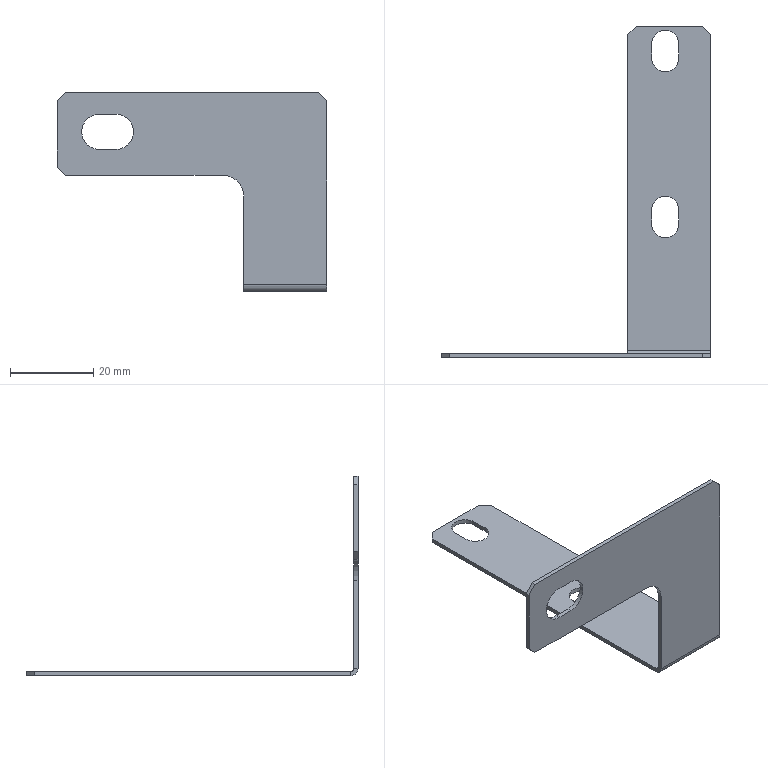Part | 1 solid | 34 faces | box 65 x 80 x 48 mm | volume 3222 mm3 | plane 25 | cylinder 9 | commonest cylinder face diameters 6.5 x4 8.5 x2 1.473 x1 3.473 x1 10 x1
STEP:
#1=CARTESIAN_POINT('',(45.,-1.,-46.263));
#2=VERTEX_POINT('',#1);
#3=CARTESIAN_POINT('',(45.,-1.,-25.));
#4=VERTEX_POINT('',#3);
#5=CARTESIAN_POINT('',(45.,-1.,-20.));
#6=DIRECTION('',(0.,0.,1.));
#7=VECTOR('',#6,1000.);
#8=LINE('',#5,#7);
#9=EDGE_CURVE('',#2,#4,#8,.T.);
#10=ORIENTED_EDGE('',*,*,#9,.T.);
#11=CARTESIAN_POINT('',(45.,0.,-25.));
#12=VERTEX_POINT('',#11);
#13=CARTESIAN_POINT('',(45.,0.,-25.));
#14=DIRECTION('',(0.,1.,0.));
#15=VECTOR('',#14,1000.);
#16=LINE('',#13,#15);
#17=EDGE_CURVE('',#4,#12,#16,.T.);
#18=ORIENTED_EDGE('',*,*,#17,.T.);
#19=CARTESIAN_POINT('',(45.,0.,-46.263));
#20=VERTEX_POINT('',#19);
#21=CARTESIAN_POINT('',(45.,0.,-20.));
#22=DIRECTION('',(0.,0.,1.));
#23=VECTOR('',#22,1000.);
#24=LINE('',#21,#23);
#25=EDGE_CURVE('',#20,#12,#24,.T.);
#26=ORIENTED_EDGE('',*,*,#25,.F.);
#27=CARTESIAN_POINT('',(45.,0.,-46.263));
#28=DIRECTION('',(0.,-1.,0.));
#29=VECTOR('',#28,1000.);
#30=LINE('',#27,#29);
#31=EDGE_CURVE('',#20,#2,#30,.T.);
#32=ORIENTED_EDGE('',*,*,#31,.T.);
#33=EDGE_LOOP('',(#10,#18,#26,#32));
#34=FACE_OUTER_BOUND('',#33,.T.);
#35=CARTESIAN_POINT('',(45.,-1.,-20.));
#36=DIRECTION('',(-1.,0.,0.));
#37=DIRECTION('',(0.,0.,1.));
#38=AXIS2_PLACEMENT_3D('',#35,#36,#37);
#39=PLANE('',#38);
#40=ADVANCED_FACE('',(#34),#39,.T.);
#41=CARTESIAN_POINT('',(10.164,-1.,-13.75));
#42=VERTEX_POINT('',#41);
#43=CARTESIAN_POINT('',(14.164,-1.,-13.75));
#44=VERTEX_POINT('',#43);
#45=CARTESIAN_POINT('',(10.164,-1.,-13.75));
#46=DIRECTION('',(1.,0.,0.));
#47=VECTOR('',#46,1000.);
#48=LINE('',#45,#47);
#49=EDGE_CURVE('',#42,#44,#48,.T.);
#50=ORIENTED_EDGE('',*,*,#49,.F.);
#51=CARTESIAN_POINT('',(10.164,-1.,-5.25));
#52=VERTEX_POINT('',#51);
#53=CARTESIAN_POINT('',(10.164,-1.,-9.5));
#54=DIRECTION('',(0.,1.,0.));
#55=DIRECTION('',(0.,0.,1.));
#56=AXIS2_PLACEMENT_3D('',#53,#54,#55);
#57=CIRCLE('',#56,4.25);
#58=EDGE_CURVE('',#42,#52,#57,.T.);
#59=ORIENTED_EDGE('',*,*,#58,.T.);
#60=CARTESIAN_POINT('',(14.164,-1.,-5.25));
#61=VERTEX_POINT('',#60);
#62=CARTESIAN_POINT('',(10.164,-1.,-5.25));
#63=DIRECTION('',(1.,0.,0.));
#64=VECTOR('',#63,1000.);
#65=LINE('',#62,#64);
#66=EDGE_CURVE('',#52,#61,#65,.T.);
#67=ORIENTED_EDGE('',*,*,#66,.T.);
#68=CARTESIAN_POINT('',(14.164,-1.,-9.5));
#69=DIRECTION('',(0.,1.,0.));
#70=DIRECTION('',(0.,0.,1.));
#71=AXIS2_PLACEMENT_3D('',#68,#69,#70);
#72=CIRCLE('',#71,4.25);
#73=EDGE_CURVE('',#61,#44,#72,.T.);
#74=ORIENTED_EDGE('',*,*,#73,.T.);
#75=EDGE_LOOP('',(#50,#59,#67,#74));
#76=FACE_BOUND('',#75,.T.);
#77=CARTESIAN_POINT('',(65.,-1.,-2.));
#78=VERTEX_POINT('',#77);
#79=CARTESIAN_POINT('',(65.,-1.,-46.263));
#80=VERTEX_POINT('',#79);
#81=CARTESIAN_POINT('',(65.,-1.,-48.));
#82=DIRECTION('',(0.,0.,-1.));
#83=VECTOR('',#82,1000.);
#84=LINE('',#81,#83);
#85=EDGE_CURVE('',#78,#80,#84,.T.);
#86=ORIENTED_EDGE('',*,*,#85,.F.);
#87=CARTESIAN_POINT('',(63.,-1.,0.));
#88=VERTEX_POINT('',#87);
#89=CARTESIAN_POINT('',(31.5,-1.,31.5));
#90=DIRECTION('',(-0.7071,0.,0.7071));
#91=VECTOR('',#90,1000.);
#92=LINE('',#89,#91);
#93=EDGE_CURVE('',#78,#88,#92,.T.);
#94=ORIENTED_EDGE('',*,*,#93,.T.);
#95=CARTESIAN_POINT('',(2.,-1.,0.));
#96=VERTEX_POINT('',#95);
#97=CARTESIAN_POINT('',(0.,-1.,0.));
#98=DIRECTION('',(1.,0.,0.));
#99=VECTOR('',#98,1000.);
#100=LINE('',#97,#99);
#101=EDGE_CURVE('',#96,#88,#100,.T.);
#102=ORIENTED_EDGE('',*,*,#101,.F.);
#103=CARTESIAN_POINT('',(0.,-1.,-2.));
#104=VERTEX_POINT('',#103);
#105=CARTESIAN_POINT('',(1.,-1.,-1.));
#106=DIRECTION('',(-0.7071,0.,-0.7071));
#107=VECTOR('',#106,1000.);
#108=LINE('',#105,#107);
#109=EDGE_CURVE('',#96,#104,#108,.T.);
#110=ORIENTED_EDGE('',*,*,#109,.T.);
#111=CARTESIAN_POINT('',(0.,-1.,-18.));
#112=VERTEX_POINT('',#111);
#113=CARTESIAN_POINT('',(0.,-1.,0.));
#114=DIRECTION('',(0.,0.,1.));
#115=VECTOR('',#114,1000.);
#116=LINE('',#113,#115);
#117=EDGE_CURVE('',#112,#104,#116,.T.);
#118=ORIENTED_EDGE('',*,*,#117,.F.);
#119=CARTESIAN_POINT('',(2.,-1.,-20.));
#120=VERTEX_POINT('',#119);
#121=CARTESIAN_POINT('',(-9.,-1.,-9.));
#122=DIRECTION('',(0.7071,0.,-0.7071));
#123=VECTOR('',#122,1000.);
#124=LINE('',#121,#123);
#125=EDGE_CURVE('',#112,#120,#124,.T.);
#126=ORIENTED_EDGE('',*,*,#125,.T.);
#127=CARTESIAN_POINT('',(40.,-1.,-20.));
#128=VERTEX_POINT('',#127);
#129=CARTESIAN_POINT('',(0.,-1.,-20.));
#130=DIRECTION('',(-1.,0.,0.));
#131=VECTOR('',#130,1000.);
#132=LINE('',#129,#131);
#133=EDGE_CURVE('',#128,#120,#132,.T.);
#134=ORIENTED_EDGE('',*,*,#133,.F.);
#135=CARTESIAN_POINT('',(40.,-1.,-25.));
#136=DIRECTION('',(0.,1.,0.));
#137=DIRECTION('',(0.,0.,-1.));
#138=AXIS2_PLACEMENT_3D('',#135,#136,#137);
#139=CIRCLE('',#138,5.);
#140=EDGE_CURVE('',#128,#4,#139,.T.);
#141=ORIENTED_EDGE('',*,*,#140,.T.);
#142=ORIENTED_EDGE('',*,*,#9,.F.);
#143=CARTESIAN_POINT('',(45.,-1.,-46.263));
#144=DIRECTION('',(1.,0.,0.));
#145=VECTOR('',#144,1000.);
#146=LINE('',#143,#145);
#147=EDGE_CURVE('',#2,#80,#146,.T.);
#148=ORIENTED_EDGE('',*,*,#147,.T.);
#149=EDGE_LOOP('',(#86,#94,#102,#110,#118,#126,#134,#141,#142,#148));
#150=FACE_OUTER_BOUND('',#149,.T.);
#151=CARTESIAN_POINT('',(0.,-1.,0.));
#152=DIRECTION('',(0.,-1.,0.));
#153=DIRECTION('',(0.,0.,-1.));
#154=AXIS2_PLACEMENT_3D('',#151,#152,#153);
#155=PLANE('',#154);
#156=ADVANCED_FACE('',(#76,#150),#155,.T.);
#157=CARTESIAN_POINT('',(10.164,0.,-13.75));
#158=VERTEX_POINT('',#157);
#159=CARTESIAN_POINT('',(10.164,0.,-5.25));
#160=VERTEX_POINT('',#159);
#161=CARTESIAN_POINT('',(10.164,0.,-9.5));
#162=DIRECTION('',(0.,1.,0.));
#163=DIRECTION('',(0.,0.,1.));
#164=AXIS2_PLACEMENT_3D('',#161,#162,#163);
#165=CIRCLE('',#164,4.25);
#166=EDGE_CURVE('',#158,#160,#165,.T.);
#167=ORIENTED_EDGE('',*,*,#166,.F.);
#168=CARTESIAN_POINT('',(14.164,0.,-13.75));
#169=VERTEX_POINT('',#168);
#170=CARTESIAN_POINT('',(10.164,0.,-13.75));
#171=DIRECTION('',(1.,0.,0.));
#172=VECTOR('',#171,1000.);
#173=LINE('',#170,#172);
#174=EDGE_CURVE('',#158,#169,#173,.T.);
#175=ORIENTED_EDGE('',*,*,#174,.T.);
#176=CARTESIAN_POINT('',(14.164,0.,-5.25));
#177=VERTEX_POINT('',#176);
#178=CARTESIAN_POINT('',(14.164,0.,-9.5));
#179=DIRECTION('',(0.,1.,0.));
#180=DIRECTION('',(0.,0.,1.));
#181=AXIS2_PLACEMENT_3D('',#178,#179,#180);
#182=CIRCLE('',#181,4.25);
#183=EDGE_CURVE('',#177,#169,#182,.T.);
#184=ORIENTED_EDGE('',*,*,#183,.F.);
#185=CARTESIAN_POINT('',(10.164,0.,-5.25));
#186=DIRECTION('',(1.,0.,0.));
#187=VECTOR('',#186,1000.);
#188=LINE('',#185,#187);
#189=EDGE_CURVE('',#160,#177,#188,.T.);
#190=ORIENTED_EDGE('',*,*,#189,.F.);
#191=EDGE_LOOP('',(#167,#175,#184,#190));
#192=FACE_BOUND('',#191,.T.);
#193=CARTESIAN_POINT('',(2.,0.,0.));
#194=VERTEX_POINT('',#193);
#195=CARTESIAN_POINT('',(63.,0.,0.));
#196=VERTEX_POINT('',#195);
#197=CARTESIAN_POINT('',(0.,0.,0.));
#198=DIRECTION('',(1.,0.,0.));
#199=VECTOR('',#198,1000.);
#200=LINE('',#197,#199);
#201=EDGE_CURVE('',#194,#196,#200,.T.);
#202=ORIENTED_EDGE('',*,*,#201,.T.);
#203=CARTESIAN_POINT('',(65.,0.,-2.));
#204=VERTEX_POINT('',#203);
#205=CARTESIAN_POINT('',(63.,0.,0.));
#206=DIRECTION('',(0.7071,0.,-0.7071));
#207=VECTOR('',#206,1000.);
#208=LINE('',#205,#207);
#209=EDGE_CURVE('',#196,#204,#208,.T.);
#210=ORIENTED_EDGE('',*,*,#209,.T.);
#211=CARTESIAN_POINT('',(65.,0.,-46.263));
#212=VERTEX_POINT('',#211);
#213=CARTESIAN_POINT('',(65.,0.,-48.));
#214=DIRECTION('',(0.,0.,-1.));
#215=VECTOR('',#214,1000.);
#216=LINE('',#213,#215);
#217=EDGE_CURVE('',#204,#212,#216,.T.);
#218=ORIENTED_EDGE('',*,*,#217,.T.);
#219=CARTESIAN_POINT('',(45.,0.,-46.263));
#220=DIRECTION('',(1.,0.,0.));
#221=VECTOR('',#220,1000.);
#222=LINE('',#219,#221);
#223=EDGE_CURVE('',#20,#212,#222,.T.);
#224=ORIENTED_EDGE('',*,*,#223,.F.);
#225=ORIENTED_EDGE('',*,*,#25,.T.);
#226=CARTESIAN_POINT('',(40.,0.,-20.));
#227=VERTEX_POINT('',#226);
#228=CARTESIAN_POINT('',(40.,0.,-25.));
#229=DIRECTION('',(0.,-1.,0.));
#230=DIRECTION('',(0.,0.,-1.));
#231=AXIS2_PLACEMENT_3D('',#228,#229,#230);
#232=CIRCLE('',#231,5.);
#233=EDGE_CURVE('',#12,#227,#232,.T.);
#234=ORIENTED_EDGE('',*,*,#233,.T.);
#235=CARTESIAN_POINT('',(2.,0.,-20.));
#236=VERTEX_POINT('',#235);
#237=CARTESIAN_POINT('',(0.,0.,-20.));
#238=DIRECTION('',(-1.,0.,0.));
#239=VECTOR('',#238,1000.);
#240=LINE('',#237,#239);
#241=EDGE_CURVE('',#227,#236,#240,.T.);
#242=ORIENTED_EDGE('',*,*,#241,.T.);
#243=CARTESIAN_POINT('',(0.,0.,-18.));
#244=VERTEX_POINT('',#243);
#245=CARTESIAN_POINT('',(2.,0.,-20.));
#246=DIRECTION('',(-0.7071,0.,0.7071));
#247=VECTOR('',#246,1000.);
#248=LINE('',#245,#247);
#249=EDGE_CURVE('',#236,#244,#248,.T.);
#250=ORIENTED_EDGE('',*,*,#249,.T.);
#251=CARTESIAN_POINT('',(0.,0.,-2.));
#252=VERTEX_POINT('',#251);
#253=CARTESIAN_POINT('',(0.,0.,0.));
#254=DIRECTION('',(0.,0.,1.));
#255=VECTOR('',#254,1000.);
#256=LINE('',#253,#255);
#257=EDGE_CURVE('',#244,#252,#256,.T.);
#258=ORIENTED_EDGE('',*,*,#257,.T.);
#259=CARTESIAN_POINT('',(0.,0.,-2.));
#260=DIRECTION('',(0.7071,0.,0.7071));
#261=VECTOR('',#260,1000.);
#262=LINE('',#259,#261);
#263=EDGE_CURVE('',#252,#194,#262,.T.);
#264=ORIENTED_EDGE('',*,*,#263,.T.);
#265=EDGE_LOOP('',(#202,#210,#218,#224,#225,#234,#242,#250,#258,#264));
#266=FACE_OUTER_BOUND('',#265,.T.);
#267=CARTESIAN_POINT('',(0.,0.,0.));
#268=DIRECTION('',(0.,-1.,0.));
#269=DIRECTION('',(0.,0.,-1.));
#270=AXIS2_PLACEMENT_3D('',#267,#268,#269);
#271=PLANE('',#270);
#272=ADVANCED_FACE('',(#192,#266),#271,.F.);
#273=ORIENTED_EDGE('',*,*,#117,.T.);
#274=CARTESIAN_POINT('',(0.,-1.,-2.));
#275=DIRECTION('',(0.,1.,0.));
#276=VECTOR('',#275,1000.);
#277=LINE('',#274,#276);
#278=EDGE_CURVE('',#104,#252,#277,.T.);
#279=ORIENTED_EDGE('',*,*,#278,.T.);
#280=ORIENTED_EDGE('',*,*,#257,.F.);
#281=CARTESIAN_POINT('',(0.,-1.,-18.));
#282=DIRECTION('',(0.,-1.,0.));
#283=VECTOR('',#282,1000.);
#284=LINE('',#281,#283);
#285=EDGE_CURVE('',#244,#112,#284,.T.);
#286=ORIENTED_EDGE('',*,*,#285,.T.);
#287=EDGE_LOOP('',(#273,#279,#280,#286));
#288=FACE_OUTER_BOUND('',#287,.T.);
#289=CARTESIAN_POINT('',(0.,-1.,0.));
#290=DIRECTION('',(-1.,0.,0.));
#291=DIRECTION('',(0.,0.,1.));
#292=AXIS2_PLACEMENT_3D('',#289,#290,#291);
#293=PLANE('',#292);
#294=ADVANCED_FACE('',(#288),#293,.T.);
#295=ORIENTED_EDGE('',*,*,#241,.F.);
#296=CARTESIAN_POINT('',(40.,-1.,-20.));
#297=DIRECTION('',(0.,-1.,0.));
#298=VECTOR('',#297,1000.);
#299=LINE('',#296,#298);
#300=EDGE_CURVE('',#227,#128,#299,.T.);
#301=ORIENTED_EDGE('',*,*,#300,.T.);
#302=ORIENTED_EDGE('',*,*,#133,.T.);
#303=CARTESIAN_POINT('',(2.,-1.,-20.));
#304=DIRECTION('',(0.,1.,0.));
#305=VECTOR('',#304,1000.);
#306=LINE('',#303,#305);
#307=EDGE_CURVE('',#120,#236,#306,.T.);
#308=ORIENTED_EDGE('',*,*,#307,.T.);
#309=EDGE_LOOP('',(#295,#301,#302,#308));
#310=FACE_OUTER_BOUND('',#309,.T.);
#311=CARTESIAN_POINT('',(0.,-1.,-20.));
#312=DIRECTION('',(0.,0.,-1.));
#313=DIRECTION('',(-1.,0.,0.));
#314=AXIS2_PLACEMENT_3D('',#311,#312,#313);
#315=PLANE('',#314);
#316=ADVANCED_FACE('',(#310),#315,.T.);
#317=ORIENTED_EDGE('',*,*,#217,.F.);
#318=CARTESIAN_POINT('',(65.,-1.,-2.));
#319=DIRECTION('',(0.,-1.,0.));
#320=VECTOR('',#319,1000.);
#321=LINE('',#318,#320);
#322=EDGE_CURVE('',#204,#78,#321,.T.);
#323=ORIENTED_EDGE('',*,*,#322,.T.);
#324=ORIENTED_EDGE('',*,*,#85,.T.);
#325=CARTESIAN_POINT('',(65.,0.,-46.263));
#326=DIRECTION('',(0.,-1.,0.));
#327=VECTOR('',#326,1000.);
#328=LINE('',#325,#327);
#329=EDGE_CURVE('',#212,#80,#328,.T.);
#330=ORIENTED_EDGE('',*,*,#329,.F.);
#331=EDGE_LOOP('',(#317,#323,#324,#330));
#332=FACE_OUTER_BOUND('',#331,.T.);
#333=CARTESIAN_POINT('',(65.,-1.,-48.));
#334=DIRECTION('',(1.,0.,0.));
#335=DIRECTION('',(0.,0.,-1.));
#336=AXIS2_PLACEMENT_3D('',#333,#334,#335);
#337=PLANE('',#336);
#338=ADVANCED_FACE('',(#332),#337,.T.);
#339=ORIENTED_EDGE('',*,*,#101,.T.);
#340=CARTESIAN_POINT('',(63.,-1.,0.));
#341=DIRECTION('',(0.,1.,0.));
#342=VECTOR('',#341,1000.);
#343=LINE('',#340,#342);
#344=EDGE_CURVE('',#88,#196,#343,.T.);
#345=ORIENTED_EDGE('',*,*,#344,.T.);
#346=ORIENTED_EDGE('',*,*,#201,.F.);
#347=CARTESIAN_POINT('',(2.,-1.,0.));
#348=DIRECTION('',(0.,-1.,0.));
#349=VECTOR('',#348,1000.);
#350=LINE('',#347,#349);
#351=EDGE_CURVE('',#194,#96,#350,.T.);
#352=ORIENTED_EDGE('',*,*,#351,.T.);
#353=EDGE_LOOP('',(#339,#345,#346,#352));
#354=FACE_OUTER_BOUND('',#353,.T.);
#355=CARTESIAN_POINT('',(0.,-1.,0.));
#356=DIRECTION('',(0.,0.,1.));
#357=DIRECTION('',(1.,0.,0.));
#358=AXIS2_PLACEMENT_3D('',#355,#356,#357);
#359=PLANE('',#358);
#360=ADVANCED_FACE('',(#354),#359,.T.);
#361=CARTESIAN_POINT('',(65.,0.7366,-47.));
#362=VERTEX_POINT('',#361);
#363=CARTESIAN_POINT('',(65.,0.7366,-48.));
#364=VERTEX_POINT('',#363);
#365=CARTESIAN_POINT('',(65.,0.7366,-48.));
#366=DIRECTION('',(0.,0.,-1.));
#367=VECTOR('',#366,1000.);
#368=LINE('',#365,#367);
#369=EDGE_CURVE('',#362,#364,#368,.T.);
#370=ORIENTED_EDGE('',*,*,#369,.F.);
#371=CARTESIAN_POINT('',(65.,0.7366,-46.263));
#372=DIRECTION('',(1.,0.,0.));
#373=DIRECTION('',(0.,0.,1.));
#374=AXIS2_PLACEMENT_3D('',#371,#372,#373);
#375=CIRCLE('',#374,0.7366);
#376=EDGE_CURVE('',#212,#362,#375,.T.);
#377=ORIENTED_EDGE('',*,*,#376,.F.);
#378=ORIENTED_EDGE('',*,*,#329,.T.);
#379=CARTESIAN_POINT('',(65.,0.7366,-46.263));
#380=DIRECTION('',(1.,0.,0.));
#381=DIRECTION('',(0.,0.,1.));
#382=AXIS2_PLACEMENT_3D('',#379,#380,#381);
#383=CIRCLE('',#382,1.737);
#384=EDGE_CURVE('',#80,#364,#383,.T.);
#385=ORIENTED_EDGE('',*,*,#384,.T.);
#386=EDGE_LOOP('',(#370,#377,#378,#385));
#387=FACE_OUTER_BOUND('',#386,.T.);
#388=CARTESIAN_POINT('',(65.,0.7366,-46.263));
#389=DIRECTION('',(1.,0.,0.));
#390=DIRECTION('',(0.,0.,-1.));
#391=AXIS2_PLACEMENT_3D('',#388,#389,#390);
#392=PLANE('',#391);
#393=ADVANCED_FACE('',(#387),#392,.T.);
#394=CARTESIAN_POINT('',(45.,0.7366,-47.));
#395=VERTEX_POINT('',#394);
#396=CARTESIAN_POINT('',(45.,0.7366,-46.263));
#397=DIRECTION('',(-1.,0.,0.));
#398=DIRECTION('',(0.,0.,1.));
#399=AXIS2_PLACEMENT_3D('',#396,#397,#398);
#400=CIRCLE('',#399,0.7366);
#401=EDGE_CURVE('',#395,#20,#400,.T.);
#402=ORIENTED_EDGE('',*,*,#401,.F.);
#403=CARTESIAN_POINT('',(45.,0.7366,-48.));
#404=VERTEX_POINT('',#403);
#405=CARTESIAN_POINT('',(45.,0.7366,-47.));
#406=DIRECTION('',(0.,0.,-1.));
#407=VECTOR('',#406,1000.);
#408=LINE('',#405,#407);
#409=EDGE_CURVE('',#395,#404,#408,.T.);
#410=ORIENTED_EDGE('',*,*,#409,.T.);
#411=CARTESIAN_POINT('',(45.,0.7366,-46.263));
#412=DIRECTION('',(-1.,0.,0.));
#413=DIRECTION('',(0.,0.,1.));
#414=AXIS2_PLACEMENT_3D('',#411,#412,#413);
#415=CIRCLE('',#414,1.737);
#416=EDGE_CURVE('',#404,#2,#415,.T.);
#417=ORIENTED_EDGE('',*,*,#416,.T.);
#418=ORIENTED_EDGE('',*,*,#31,.F.);
#419=EDGE_LOOP('',(#402,#410,#417,#418));
#420=FACE_OUTER_BOUND('',#419,.T.);
#421=CARTESIAN_POINT('',(45.,0.7366,-46.263));
#422=DIRECTION('',(1.,0.,0.));
#423=DIRECTION('',(0.,0.,-1.));
#424=AXIS2_PLACEMENT_3D('',#421,#422,#423);
#425=PLANE('',#424);
#426=ADVANCED_FACE('',(#420),#425,.F.);
#427=ORIENTED_EDGE('',*,*,#147,.F.);
#428=ORIENTED_EDGE('',*,*,#416,.F.);
#429=CARTESIAN_POINT('',(0.,0.7366,-48.));
#430=DIRECTION('',(-1.,0.,0.));
#431=VECTOR('',#430,1000.);
#432=LINE('',#429,#431);
#433=EDGE_CURVE('',#364,#404,#432,.T.);
#434=ORIENTED_EDGE('',*,*,#433,.F.);
#435=ORIENTED_EDGE('',*,*,#384,.F.);
#436=EDGE_LOOP('',(#427,#428,#434,#435));
#437=FACE_OUTER_BOUND('',#436,.T.);
#438=CARTESIAN_POINT('',(45.,0.7366,-46.263));
#439=DIRECTION('',(-1.,0.,0.));
#440=DIRECTION('',(0.,0.,-1.));
#441=AXIS2_PLACEMENT_3D('',#438,#439,#440);
#442=CYLINDRICAL_SURFACE('',#441,1.737);
#443=ADVANCED_FACE('',(#437),#442,.T.);
#444=ORIENTED_EDGE('',*,*,#223,.T.);
#445=ORIENTED_EDGE('',*,*,#376,.T.);
#446=CARTESIAN_POINT('',(65.,0.7366,-47.));
#447=DIRECTION('',(-1.,0.,0.));
#448=VECTOR('',#447,1000.);
#449=LINE('',#446,#448);
#450=EDGE_CURVE('',#362,#395,#449,.T.);
#451=ORIENTED_EDGE('',*,*,#450,.T.);
#452=ORIENTED_EDGE('',*,*,#401,.T.);
#453=EDGE_LOOP('',(#444,#445,#451,#452));
#454=FACE_OUTER_BOUND('',#453,.T.);
#455=CARTESIAN_POINT('',(45.,0.7366,-46.263));
#456=DIRECTION('',(-1.,0.,0.));
#457=DIRECTION('',(0.,0.,-1.));
#458=AXIS2_PLACEMENT_3D('',#455,#456,#457);
#459=CYLINDRICAL_SURFACE('',#458,0.7366);
#460=ADVANCED_FACE('',(#454),#459,.F.);
#461=CARTESIAN_POINT('',(45.,77.,-47.));
#462=VERTEX_POINT('',#461);
#463=CARTESIAN_POINT('',(45.,0.,-47.));
#464=DIRECTION('',(0.,-1.,0.));
#465=VECTOR('',#464,1000.);
#466=LINE('',#463,#465);
#467=EDGE_CURVE('',#462,#395,#466,.T.);
#468=ORIENTED_EDGE('',*,*,#467,.F.);
#469=CARTESIAN_POINT('',(45.,77.,-48.));
#470=VERTEX_POINT('',#469);
#471=CARTESIAN_POINT('',(45.,77.,-48.));
#472=DIRECTION('',(0.,0.,-1.));
#473=VECTOR('',#472,1000.);
#474=LINE('',#471,#473);
#475=EDGE_CURVE('',#462,#470,#474,.T.);
#476=ORIENTED_EDGE('',*,*,#475,.T.);
#477=CARTESIAN_POINT('',(45.,0.,-48.));
#478=DIRECTION('',(0.,-1.,0.));
#479=VECTOR('',#478,1000.);
#480=LINE('',#477,#479);
#481=EDGE_CURVE('',#470,#404,#480,.T.);
#482=ORIENTED_EDGE('',*,*,#481,.T.);
#483=ORIENTED_EDGE('',*,*,#409,.F.);
#484=EDGE_LOOP('',(#468,#476,#482,#483));
#485=FACE_OUTER_BOUND('',#484,.T.);
#486=CARTESIAN_POINT('',(45.,0.,-48.));
#487=DIRECTION('',(-1.,0.,0.));
#488=DIRECTION('',(0.,0.,1.));
#489=AXIS2_PLACEMENT_3D('',#486,#487,#488);
#490=PLANE('',#489);
#491=ADVANCED_FACE('',(#485),#490,.T.);
#492=CARTESIAN_POINT('',(65.,77.,-48.));
#493=VERTEX_POINT('',#492);
#494=CARTESIAN_POINT('',(65.,79.,-48.));
#495=DIRECTION('',(0.,1.,0.));
#496=VECTOR('',#495,1000.);
#497=LINE('',#494,#496);
#498=EDGE_CURVE('',#364,#493,#497,.T.);
#499=ORIENTED_EDGE('',*,*,#498,.T.);
#500=CARTESIAN_POINT('',(65.,77.,-47.));
#501=VERTEX_POINT('',#500);
#502=CARTESIAN_POINT('',(65.,77.,-48.));
#503=DIRECTION('',(0.,0.,1.));
#504=VECTOR('',#503,1000.);
#505=LINE('',#502,#504);
#506=EDGE_CURVE('',#493,#501,#505,.T.);
#507=ORIENTED_EDGE('',*,*,#506,.T.);
#508=CARTESIAN_POINT('',(65.,0.,-47.));
#509=DIRECTION('',(0.,1.,0.));
#510=VECTOR('',#509,1000.);
#511=LINE('',#508,#510);
#512=EDGE_CURVE('',#362,#501,#511,.T.);
#513=ORIENTED_EDGE('',*,*,#512,.F.);
#514=ORIENTED_EDGE('',*,*,#369,.T.);
#515=EDGE_LOOP('',(#499,#507,#513,#514));
#516=FACE_OUTER_BOUND('',#515,.T.);
#517=CARTESIAN_POINT('',(65.,79.,-48.));
#518=DIRECTION('',(1.,0.,0.));
#519=DIRECTION('',(0.,1.,0.));
#520=AXIS2_PLACEMENT_3D('',#517,#518,#519);
#521=PLANE('',#520);
#522=ADVANCED_FACE('',(#516),#521,.T.);
#523=CARTESIAN_POINT('',(50.75,71.25,-48.));
#524=VERTEX_POINT('',#523);
#525=CARTESIAN_POINT('',(50.75,74.75,-48.));
#526=VERTEX_POINT('',#525);
#527=CARTESIAN_POINT('',(50.75,71.25,-48.));
#528=DIRECTION('',(0.,1.,0.));
#529=VECTOR('',#528,1000.);
#530=LINE('',#527,#529);
#531=EDGE_CURVE('',#524,#526,#530,.T.);
#532=ORIENTED_EDGE('',*,*,#531,.F.);
#533=CARTESIAN_POINT('',(57.25,71.25,-48.));
#534=VERTEX_POINT('',#533);
#535=CARTESIAN_POINT('',(54.,71.25,-48.));
#536=DIRECTION('',(0.,0.,1.));
#537=DIRECTION('',(1.,0.,0.));
#538=AXIS2_PLACEMENT_3D('',#535,#536,#537);
#539=CIRCLE('',#538,3.25);
#540=EDGE_CURVE('',#524,#534,#539,.T.);
#541=ORIENTED_EDGE('',*,*,#540,.T.);
#542=CARTESIAN_POINT('',(57.25,74.75,-48.));
#543=VERTEX_POINT('',#542);
#544=CARTESIAN_POINT('',(57.25,71.25,-48.));
#545=DIRECTION('',(0.,1.,0.));
#546=VECTOR('',#545,1000.);
#547=LINE('',#544,#546);
#548=EDGE_CURVE('',#534,#543,#547,.T.);
#549=ORIENTED_EDGE('',*,*,#548,.T.);
#550=CARTESIAN_POINT('',(54.,74.75,-48.));
#551=DIRECTION('',(0.,0.,1.));
#552=DIRECTION('',(1.,0.,0.));
#553=AXIS2_PLACEMENT_3D('',#550,#551,#552);
#554=CIRCLE('',#553,3.25);
#555=EDGE_CURVE('',#543,#526,#554,.T.);
#556=ORIENTED_EDGE('',*,*,#555,.T.);
#557=EDGE_LOOP('',(#532,#541,#549,#556));
#558=FACE_BOUND('',#557,.T.);
#559=CARTESIAN_POINT('',(50.75,31.25,-48.));
#560=VERTEX_POINT('',#559);
#561=CARTESIAN_POINT('',(50.75,34.75,-48.));
#562=VERTEX_POINT('',#561);
#563=CARTESIAN_POINT('',(50.75,31.25,-48.));
#564=DIRECTION('',(0.,1.,0.));
#565=VECTOR('',#564,1000.);
#566=LINE('',#563,#565);
#567=EDGE_CURVE('',#560,#562,#566,.T.);
#568=ORIENTED_EDGE('',*,*,#567,.F.);
#569=CARTESIAN_POINT('',(57.25,31.25,-48.));
#570=VERTEX_POINT('',#569);
#571=CARTESIAN_POINT('',(54.,31.25,-48.));
#572=DIRECTION('',(0.,0.,1.));
#573=DIRECTION('',(1.,0.,0.));
#574=AXIS2_PLACEMENT_3D('',#571,#572,#573);
#575=CIRCLE('',#574,3.25);
#576=EDGE_CURVE('',#560,#570,#575,.T.);
#577=ORIENTED_EDGE('',*,*,#576,.T.);
#578=CARTESIAN_POINT('',(57.25,34.75,-48.));
#579=VERTEX_POINT('',#578);
#580=CARTESIAN_POINT('',(57.25,31.25,-48.));
#581=DIRECTION('',(0.,1.,0.));
#582=VECTOR('',#581,1000.);
#583=LINE('',#580,#582);
#584=EDGE_CURVE('',#570,#579,#583,.T.);
#585=ORIENTED_EDGE('',*,*,#584,.T.);
#586=CARTESIAN_POINT('',(54.,34.75,-48.));
#587=DIRECTION('',(0.,0.,1.));
#588=DIRECTION('',(1.,0.,0.));
#589=AXIS2_PLACEMENT_3D('',#586,#587,#588);
#590=CIRCLE('',#589,3.25);
#591=EDGE_CURVE('',#579,#562,#590,.T.);
#592=ORIENTED_EDGE('',*,*,#591,.T.);
#593=EDGE_LOOP('',(#568,#577,#585,#592));
#594=FACE_BOUND('',#593,.T.);
#595=ORIENTED_EDGE('',*,*,#481,.F.);
#596=CARTESIAN_POINT('',(47.,79.,-48.));
#597=VERTEX_POINT('',#596);
#598=CARTESIAN_POINT('',(-16.,16.,-48.));
#599=DIRECTION('',(0.7071,0.7071,0.));
#600=VECTOR('',#599,1000.);
#601=LINE('',#598,#600);
#602=EDGE_CURVE('',#470,#597,#601,.T.);
#603=ORIENTED_EDGE('',*,*,#602,.T.);
#604=CARTESIAN_POINT('',(63.,79.,-48.));
#605=VERTEX_POINT('',#604);
#606=CARTESIAN_POINT('',(45.,79.,-48.));
#607=DIRECTION('',(-1.,0.,0.));
#608=VECTOR('',#607,1000.);
#609=LINE('',#606,#608);
#610=EDGE_CURVE('',#605,#597,#609,.T.);
#611=ORIENTED_EDGE('',*,*,#610,.F.);
#612=CARTESIAN_POINT('',(71.,71.,-48.));
#613=DIRECTION('',(0.7071,-0.7071,0.));
#614=VECTOR('',#613,1000.);
#615=LINE('',#612,#614);
#616=EDGE_CURVE('',#605,#493,#615,.T.);
#617=ORIENTED_EDGE('',*,*,#616,.T.);
#618=ORIENTED_EDGE('',*,*,#498,.F.);
#619=ORIENTED_EDGE('',*,*,#433,.T.);
#620=EDGE_LOOP('',(#595,#603,#611,#617,#618,#619));
#621=FACE_OUTER_BOUND('',#620,.T.);
#622=CARTESIAN_POINT('',(0.,0.,-48.));
#623=DIRECTION('',(0.,0.,-1.));
#624=DIRECTION('',(-1.,0.,0.));
#625=AXIS2_PLACEMENT_3D('',#622,#623,#624);
#626=PLANE('',#625);
#627=ADVANCED_FACE('',(#558,#594,#621),#626,.T.);
#628=CARTESIAN_POINT('',(50.75,71.25,-47.));
#629=VERTEX_POINT('',#628);
#630=CARTESIAN_POINT('',(57.25,71.25,-47.));
#631=VERTEX_POINT('',#630);
#632=CARTESIAN_POINT('',(54.,71.25,-47.));
#633=DIRECTION('',(0.,0.,1.));
#634=DIRECTION('',(1.,0.,0.));
#635=AXIS2_PLACEMENT_3D('',#632,#633,#634);
#636=CIRCLE('',#635,3.25);
#637=EDGE_CURVE('',#629,#631,#636,.T.);
#638=ORIENTED_EDGE('',*,*,#637,.F.);
#639=CARTESIAN_POINT('',(50.75,74.75,-47.));
#640=VERTEX_POINT('',#639);
#641=CARTESIAN_POINT('',(50.75,71.25,-47.));
#642=DIRECTION('',(0.,1.,0.));
#643=VECTOR('',#642,1000.);
#644=LINE('',#641,#643);
#645=EDGE_CURVE('',#629,#640,#644,.T.);
#646=ORIENTED_EDGE('',*,*,#645,.T.);
#647=CARTESIAN_POINT('',(57.25,74.75,-47.));
#648=VERTEX_POINT('',#647);
#649=CARTESIAN_POINT('',(54.,74.75,-47.));
#650=DIRECTION('',(0.,0.,1.));
#651=DIRECTION('',(1.,0.,0.));
#652=AXIS2_PLACEMENT_3D('',#649,#650,#651);
#653=CIRCLE('',#652,3.25);
#654=EDGE_CURVE('',#648,#640,#653,.T.);
#655=ORIENTED_EDGE('',*,*,#654,.F.);
#656=CARTESIAN_POINT('',(57.25,71.25,-47.));
#657=DIRECTION('',(0.,1.,0.));
#658=VECTOR('',#657,1000.);
#659=LINE('',#656,#658);
#660=EDGE_CURVE('',#631,#648,#659,.T.);
#661=ORIENTED_EDGE('',*,*,#660,.F.);
#662=EDGE_LOOP('',(#638,#646,#655,#661));
#663=FACE_BOUND('',#662,.T.);
#664=CARTESIAN_POINT('',(50.75,31.25,-47.));
#665=VERTEX_POINT('',#664);
#666=CARTESIAN_POINT('',(57.25,31.25,-47.));
#667=VERTEX_POINT('',#666);
#668=CARTESIAN_POINT('',(54.,31.25,-47.));
#669=DIRECTION('',(0.,0.,1.));
#670=DIRECTION('',(1.,0.,0.));
#671=AXIS2_PLACEMENT_3D('',#668,#669,#670);
#672=CIRCLE('',#671,3.25);
#673=EDGE_CURVE('',#665,#667,#672,.T.);
#674=ORIENTED_EDGE('',*,*,#673,.F.);
#675=CARTESIAN_POINT('',(50.75,34.75,-47.));
#676=VERTEX_POINT('',#675);
#677=CARTESIAN_POINT('',(50.75,31.25,-47.));
#678=DIRECTION('',(0.,1.,0.));
#679=VECTOR('',#678,1000.);
#680=LINE('',#677,#679);
#681=EDGE_CURVE('',#665,#676,#680,.T.);
#682=ORIENTED_EDGE('',*,*,#681,.T.);
#683=CARTESIAN_POINT('',(57.25,34.75,-47.));
#684=VERTEX_POINT('',#683);
#685=CARTESIAN_POINT('',(54.,34.75,-47.));
#686=DIRECTION('',(0.,0.,1.));
#687=DIRECTION('',(1.,0.,0.));
#688=AXIS2_PLACEMENT_3D('',#685,#686,#687);
#689=CIRCLE('',#688,3.25);
#690=EDGE_CURVE('',#684,#676,#689,.T.);
#691=ORIENTED_EDGE('',*,*,#690,.F.);
#692=CARTESIAN_POINT('',(57.25,31.25,-47.));
#693=DIRECTION('',(0.,1.,0.));
#694=VECTOR('',#693,1000.);
#695=LINE('',#692,#694);
#696=EDGE_CURVE('',#667,#684,#695,.T.);
#697=ORIENTED_EDGE('',*,*,#696,.F.);
#698=EDGE_LOOP('',(#674,#682,#691,#697));
#699=FACE_BOUND('',#698,.T.);
#700=CARTESIAN_POINT('',(63.,79.,-47.));
#701=VERTEX_POINT('',#700);
#702=CARTESIAN_POINT('',(47.,79.,-47.));
#703=VERTEX_POINT('',#702);
#704=CARTESIAN_POINT('',(0.,79.,-47.));
#705=DIRECTION('',(-1.,0.,0.));
#706=VECTOR('',#705,1000.);
#707=LINE('',#704,#706);
#708=EDGE_CURVE('',#701,#703,#707,.T.);
#709=ORIENTED_EDGE('',*,*,#708,.T.);
#710=CARTESIAN_POINT('',(47.,79.,-47.));
#711=DIRECTION('',(-0.7071,-0.7071,0.));
#712=VECTOR('',#711,1000.);
#713=LINE('',#710,#712);
#714=EDGE_CURVE('',#703,#462,#713,.T.);
#715=ORIENTED_EDGE('',*,*,#714,.T.);
#716=ORIENTED_EDGE('',*,*,#467,.T.);
#717=ORIENTED_EDGE('',*,*,#450,.F.);
#718=ORIENTED_EDGE('',*,*,#512,.T.);
#719=CARTESIAN_POINT('',(65.,77.,-47.));
#720=DIRECTION('',(-0.7071,0.7071,0.));
#721=VECTOR('',#720,1000.);
#722=LINE('',#719,#721);
#723=EDGE_CURVE('',#501,#701,#722,.T.);
#724=ORIENTED_EDGE('',*,*,#723,.T.);
#725=EDGE_LOOP('',(#709,#715,#716,#717,#718,#724));
#726=FACE_OUTER_BOUND('',#725,.T.);
#727=CARTESIAN_POINT('',(0.,0.,-47.));
#728=DIRECTION('',(0.,0.,-1.));
#729=DIRECTION('',(-1.,0.,0.));
#730=AXIS2_PLACEMENT_3D('',#727,#728,#729);
#731=PLANE('',#730);
#732=ADVANCED_FACE('',(#663,#699,#726),#731,.F.);
#733=ORIENTED_EDGE('',*,*,#610,.T.);
#734=CARTESIAN_POINT('',(47.,79.,-48.));
#735=DIRECTION('',(0.,0.,1.));
#736=VECTOR('',#735,1000.);
#737=LINE('',#734,#736);
#738=EDGE_CURVE('',#597,#703,#737,.T.);
#739=ORIENTED_EDGE('',*,*,#738,.T.);
#740=ORIENTED_EDGE('',*,*,#708,.F.);
#741=CARTESIAN_POINT('',(63.,79.,-48.));
#742=DIRECTION('',(0.,0.,-1.));
#743=VECTOR('',#742,1000.);
#744=LINE('',#741,#743);
#745=EDGE_CURVE('',#701,#605,#744,.T.);
#746=ORIENTED_EDGE('',*,*,#745,.T.);
#747=EDGE_LOOP('',(#733,#739,#740,#746));
#748=FACE_OUTER_BOUND('',#747,.T.);
#749=CARTESIAN_POINT('',(45.,79.,-48.));
#750=DIRECTION('',(0.,1.,0.));
#751=DIRECTION('',(0.,0.,1.));
#752=AXIS2_PLACEMENT_3D('',#749,#750,#751);
#753=PLANE('',#752);
#754=ADVANCED_FACE('',(#748),#753,.T.);
#755=ORIENTED_EDGE('',*,*,#73,.F.);
#756=CARTESIAN_POINT('',(14.164,0.,-5.25));
#757=DIRECTION('',(0.,-1.,0.));
#758=VECTOR('',#757,1000.);
#759=LINE('',#756,#758);
#760=EDGE_CURVE('',#177,#61,#759,.T.);
#761=ORIENTED_EDGE('',*,*,#760,.F.);
#762=ORIENTED_EDGE('',*,*,#183,.T.);
#763=CARTESIAN_POINT('',(14.164,0.,-13.75));
#764=DIRECTION('',(0.,1.,0.));
#765=VECTOR('',#764,1000.);
#766=LINE('',#763,#765);
#767=EDGE_CURVE('',#44,#169,#766,.T.);
#768=ORIENTED_EDGE('',*,*,#767,.F.);
#769=EDGE_LOOP('',(#755,#761,#762,#768));
#770=FACE_OUTER_BOUND('',#769,.T.);
#771=CARTESIAN_POINT('',(14.164,0.,-9.5));
#772=DIRECTION('',(0.,1.,0.));
#773=DIRECTION('',(0.,0.,1.));
#774=AXIS2_PLACEMENT_3D('',#771,#772,#773);
#775=CYLINDRICAL_SURFACE('',#774,4.25);
#776=ADVANCED_FACE('',(#770),#775,.F.);
#777=ORIENTED_EDGE('',*,*,#166,.T.);
#778=CARTESIAN_POINT('',(10.164,0.,-5.25));
#779=DIRECTION('',(0.,1.,0.));
#780=VECTOR('',#779,1000.);
#781=LINE('',#778,#780);
#782=EDGE_CURVE('',#52,#160,#781,.T.);
#783=ORIENTED_EDGE('',*,*,#782,.F.);
#784=ORIENTED_EDGE('',*,*,#58,.F.);
#785=CARTESIAN_POINT('',(10.164,0.,-13.75));
#786=DIRECTION('',(0.,-1.,0.));
#787=VECTOR('',#786,1000.);
#788=LINE('',#785,#787);
#789=EDGE_CURVE('',#158,#42,#788,.T.);
#790=ORIENTED_EDGE('',*,*,#789,.F.);
#791=EDGE_LOOP('',(#777,#783,#784,#790));
#792=FACE_OUTER_BOUND('',#791,.T.);
#793=CARTESIAN_POINT('',(10.164,0.,-9.5));
#794=DIRECTION('',(0.,1.,0.));
#795=DIRECTION('',(0.,0.,1.));
#796=AXIS2_PLACEMENT_3D('',#793,#794,#795);
#797=CYLINDRICAL_SURFACE('',#796,4.25);
#798=ADVANCED_FACE('',(#792),#797,.F.);
#799=ORIENTED_EDGE('',*,*,#767,.T.);
#800=ORIENTED_EDGE('',*,*,#174,.F.);
#801=ORIENTED_EDGE('',*,*,#789,.T.);
#802=ORIENTED_EDGE('',*,*,#49,.T.);
#803=EDGE_LOOP('',(#799,#800,#801,#802));
#804=FACE_OUTER_BOUND('',#803,.T.);
#805=CARTESIAN_POINT('',(10.164,0.,-13.75));
#806=DIRECTION('',(0.,0.,-1.));
#807=DIRECTION('',(-1.,0.,0.));
#808=AXIS2_PLACEMENT_3D('',#805,#806,#807);
#809=PLANE('',#808);
#810=ADVANCED_FACE('',(#804),#809,.F.);
#811=ORIENTED_EDGE('',*,*,#760,.T.);
#812=ORIENTED_EDGE('',*,*,#66,.F.);
#813=ORIENTED_EDGE('',*,*,#782,.T.);
#814=ORIENTED_EDGE('',*,*,#189,.T.);
#815=EDGE_LOOP('',(#811,#812,#813,#814));
#816=FACE_OUTER_BOUND('',#815,.T.);
#817=CARTESIAN_POINT('',(10.164,0.,-5.25));
#818=DIRECTION('',(0.,0.,1.));
#819=DIRECTION('',(1.,0.,0.));
#820=AXIS2_PLACEMENT_3D('',#817,#818,#819);
#821=PLANE('',#820);
#822=ADVANCED_FACE('',(#816),#821,.F.);
#823=ORIENTED_EDGE('',*,*,#591,.F.);
#824=CARTESIAN_POINT('',(57.25,34.75,-48.));
#825=DIRECTION('',(0.,0.,-1.));
#826=VECTOR('',#825,1000.);
#827=LINE('',#824,#826);
#828=EDGE_CURVE('',#684,#579,#827,.T.);
#829=ORIENTED_EDGE('',*,*,#828,.F.);
#830=ORIENTED_EDGE('',*,*,#690,.T.);
#831=CARTESIAN_POINT('',(50.75,34.75,-47.));
#832=DIRECTION('',(0.,0.,1.));
#833=VECTOR('',#832,1000.);
#834=LINE('',#831,#833);
#835=EDGE_CURVE('',#562,#676,#834,.T.);
#836=ORIENTED_EDGE('',*,*,#835,.F.);
#837=EDGE_LOOP('',(#823,#829,#830,#836));
#838=FACE_OUTER_BOUND('',#837,.T.);
#839=CARTESIAN_POINT('',(54.,34.75,-47.));
#840=DIRECTION('',(0.,0.,1.));
#841=DIRECTION('',(1.,0.,0.));
#842=AXIS2_PLACEMENT_3D('',#839,#840,#841);
#843=CYLINDRICAL_SURFACE('',#842,3.25);
#844=ADVANCED_FACE('',(#838),#843,.F.);
#845=ORIENTED_EDGE('',*,*,#673,.T.);
#846=CARTESIAN_POINT('',(57.25,31.25,-48.));
#847=DIRECTION('',(0.,0.,-1.));
#848=VECTOR('',#847,1000.);
#849=LINE('',#846,#848);
#850=EDGE_CURVE('',#667,#570,#849,.T.);
#851=ORIENTED_EDGE('',*,*,#850,.T.);
#852=ORIENTED_EDGE('',*,*,#576,.F.);
#853=CARTESIAN_POINT('',(50.75,31.25,-47.));
#854=DIRECTION('',(0.,0.,-1.));
#855=VECTOR('',#854,1000.);
#856=LINE('',#853,#855);
#857=EDGE_CURVE('',#665,#560,#856,.T.);
#858=ORIENTED_EDGE('',*,*,#857,.F.);
#859=EDGE_LOOP('',(#845,#851,#852,#858));
#860=FACE_OUTER_BOUND('',#859,.T.);
#861=CARTESIAN_POINT('',(54.,31.25,-47.));
#862=DIRECTION('',(0.,0.,1.));
#863=DIRECTION('',(1.,0.,0.));
#864=AXIS2_PLACEMENT_3D('',#861,#862,#863);
#865=CYLINDRICAL_SURFACE('',#864,3.25);
#866=ADVANCED_FACE('',(#860),#865,.F.);
#867=ORIENTED_EDGE('',*,*,#835,.T.);
#868=ORIENTED_EDGE('',*,*,#681,.F.);
#869=ORIENTED_EDGE('',*,*,#857,.T.);
#870=ORIENTED_EDGE('',*,*,#567,.T.);
#871=EDGE_LOOP('',(#867,#868,#869,#870));
#872=FACE_OUTER_BOUND('',#871,.T.);
#873=CARTESIAN_POINT('',(50.75,31.25,-47.));
#874=DIRECTION('',(-1.,0.,0.));
#875=DIRECTION('',(0.,0.,1.));
#876=AXIS2_PLACEMENT_3D('',#873,#874,#875);
#877=PLANE('',#876);
#878=ADVANCED_FACE('',(#872),#877,.F.);
#879=ORIENTED_EDGE('',*,*,#828,.T.);
#880=ORIENTED_EDGE('',*,*,#584,.F.);
#881=ORIENTED_EDGE('',*,*,#850,.F.);
#882=ORIENTED_EDGE('',*,*,#696,.T.);
#883=EDGE_LOOP('',(#879,#880,#881,#882));
#884=FACE_OUTER_BOUND('',#883,.T.);
#885=CARTESIAN_POINT('',(57.25,31.25,-48.));
#886=DIRECTION('',(1.,0.,0.));
#887=DIRECTION('',(0.,0.,-1.));
#888=AXIS2_PLACEMENT_3D('',#885,#886,#887);
#889=PLANE('',#888);
#890=ADVANCED_FACE('',(#884),#889,.F.);
#891=ORIENTED_EDGE('',*,*,#555,.F.);
#892=CARTESIAN_POINT('',(57.25,74.75,-48.));
#893=DIRECTION('',(0.,0.,-1.));
#894=VECTOR('',#893,1000.);
#895=LINE('',#892,#894);
#896=EDGE_CURVE('',#648,#543,#895,.T.);
#897=ORIENTED_EDGE('',*,*,#896,.F.);
#898=ORIENTED_EDGE('',*,*,#654,.T.);
#899=CARTESIAN_POINT('',(50.75,74.75,-47.));
#900=DIRECTION('',(0.,0.,1.));
#901=VECTOR('',#900,1000.);
#902=LINE('',#899,#901);
#903=EDGE_CURVE('',#526,#640,#902,.T.);
#904=ORIENTED_EDGE('',*,*,#903,.F.);
#905=EDGE_LOOP('',(#891,#897,#898,#904));
#906=FACE_OUTER_BOUND('',#905,.T.);
#907=CARTESIAN_POINT('',(54.,74.75,-47.));
#908=DIRECTION('',(0.,0.,1.));
#909=DIRECTION('',(1.,0.,0.));
#910=AXIS2_PLACEMENT_3D('',#907,#908,#909);
#911=CYLINDRICAL_SURFACE('',#910,3.25);
#912=ADVANCED_FACE('',(#906),#911,.F.);
#913=ORIENTED_EDGE('',*,*,#637,.T.);
#914=CARTESIAN_POINT('',(57.25,71.25,-48.));
#915=DIRECTION('',(0.,0.,-1.));
#916=VECTOR('',#915,1000.);
#917=LINE('',#914,#916);
#918=EDGE_CURVE('',#631,#534,#917,.T.);
#919=ORIENTED_EDGE('',*,*,#918,.T.);
#920=ORIENTED_EDGE('',*,*,#540,.F.);
#921=CARTESIAN_POINT('',(50.75,71.25,-47.));
#922=DIRECTION('',(0.,0.,-1.));
#923=VECTOR('',#922,1000.);
#924=LINE('',#921,#923);
#925=EDGE_CURVE('',#629,#524,#924,.T.);
#926=ORIENTED_EDGE('',*,*,#925,.F.);
#927=EDGE_LOOP('',(#913,#919,#920,#926));
#928=FACE_OUTER_BOUND('',#927,.T.);
#929=CARTESIAN_POINT('',(54.,71.25,-47.));
#930=DIRECTION('',(0.,0.,1.));
#931=DIRECTION('',(1.,0.,0.));
#932=AXIS2_PLACEMENT_3D('',#929,#930,#931);
#933=CYLINDRICAL_SURFACE('',#932,3.25);
#934=ADVANCED_FACE('',(#928),#933,.F.);
#935=ORIENTED_EDGE('',*,*,#903,.T.);
#936=ORIENTED_EDGE('',*,*,#645,.F.);
#937=ORIENTED_EDGE('',*,*,#925,.T.);
#938=ORIENTED_EDGE('',*,*,#531,.T.);
#939=EDGE_LOOP('',(#935,#936,#937,#938));
#940=FACE_OUTER_BOUND('',#939,.T.);
#941=CARTESIAN_POINT('',(50.75,71.25,-47.));
#942=DIRECTION('',(-1.,0.,0.));
#943=DIRECTION('',(0.,0.,1.));
#944=AXIS2_PLACEMENT_3D('',#941,#942,#943);
#945=PLANE('',#944);
#946=ADVANCED_FACE('',(#940),#945,.F.);
#947=ORIENTED_EDGE('',*,*,#896,.T.);
#948=ORIENTED_EDGE('',*,*,#548,.F.);
#949=ORIENTED_EDGE('',*,*,#918,.F.);
#950=ORIENTED_EDGE('',*,*,#660,.T.);
#951=EDGE_LOOP('',(#947,#948,#949,#950));
#952=FACE_OUTER_BOUND('',#951,.T.);
#953=CARTESIAN_POINT('',(57.25,71.25,-48.));
#954=DIRECTION('',(1.,0.,0.));
#955=DIRECTION('',(0.,0.,-1.));
#956=AXIS2_PLACEMENT_3D('',#953,#954,#955);
#957=PLANE('',#956);
#958=ADVANCED_FACE('',(#952),#957,.F.);
#959=ORIENTED_EDGE('',*,*,#125,.F.);
#960=ORIENTED_EDGE('',*,*,#285,.F.);
#961=ORIENTED_EDGE('',*,*,#249,.F.);
#962=ORIENTED_EDGE('',*,*,#307,.F.);
#963=EDGE_LOOP('',(#959,#960,#961,#962));
#964=FACE_OUTER_BOUND('',#963,.T.);
#965=CARTESIAN_POINT('',(2.,-1.,-20.));
#966=DIRECTION('',(0.7071,0.,0.7071));
#967=DIRECTION('',(0.,1.,0.));
#968=AXIS2_PLACEMENT_3D('',#965,#966,#967);
#969=PLANE('',#968);
#970=ADVANCED_FACE('',(#964),#969,.F.);
#971=ORIENTED_EDGE('',*,*,#109,.F.);
#972=ORIENTED_EDGE('',*,*,#351,.F.);
#973=ORIENTED_EDGE('',*,*,#263,.F.);
#974=ORIENTED_EDGE('',*,*,#278,.F.);
#975=EDGE_LOOP('',(#971,#972,#973,#974));
#976=FACE_OUTER_BOUND('',#975,.T.);
#977=CARTESIAN_POINT('',(0.,-1.,-2.));
#978=DIRECTION('',(0.7071,0.,-0.7071));
#979=DIRECTION('',(0.,1.,0.));
#980=AXIS2_PLACEMENT_3D('',#977,#978,#979);
#981=PLANE('',#980);
#982=ADVANCED_FACE('',(#976),#981,.F.);
#983=ORIENTED_EDGE('',*,*,#93,.F.);
#984=ORIENTED_EDGE('',*,*,#322,.F.);
#985=ORIENTED_EDGE('',*,*,#209,.F.);
#986=ORIENTED_EDGE('',*,*,#344,.F.);
#987=EDGE_LOOP('',(#983,#984,#985,#986));
#988=FACE_OUTER_BOUND('',#987,.T.);
#989=CARTESIAN_POINT('',(63.,-1.,0.));
#990=DIRECTION('',(-0.7071,0.,-0.7071));
#991=DIRECTION('',(0.,1.,0.));
#992=AXIS2_PLACEMENT_3D('',#989,#990,#991);
#993=PLANE('',#992);
#994=ADVANCED_FACE('',(#988),#993,.F.);
#995=ORIENTED_EDGE('',*,*,#616,.F.);
#996=ORIENTED_EDGE('',*,*,#745,.F.);
#997=ORIENTED_EDGE('',*,*,#723,.F.);
#998=ORIENTED_EDGE('',*,*,#506,.F.);
#999=EDGE_LOOP('',(#995,#996,#997,#998));
#1000=FACE_OUTER_BOUND('',#999,.T.);
#1001=CARTESIAN_POINT('',(65.,77.,-48.));
#1002=DIRECTION('',(-0.7071,-0.7071,0.));
#1003=DIRECTION('',(0.,0.,1.));
#1004=AXIS2_PLACEMENT_3D('',#1001,#1002,#1003);
#1005=PLANE('',#1004);
#1006=ADVANCED_FACE('',(#1000),#1005,.F.);
#1007=ORIENTED_EDGE('',*,*,#602,.F.);
#1008=ORIENTED_EDGE('',*,*,#475,.F.);
#1009=ORIENTED_EDGE('',*,*,#714,.F.);
#1010=ORIENTED_EDGE('',*,*,#738,.F.);
#1011=EDGE_LOOP('',(#1007,#1008,#1009,#1010));
#1012=FACE_OUTER_BOUND('',#1011,.T.);
#1013=CARTESIAN_POINT('',(47.,79.,-48.));
#1014=DIRECTION('',(0.7071,-0.7071,0.));
#1015=DIRECTION('',(0.,0.,1.));
#1016=AXIS2_PLACEMENT_3D('',#1013,#1014,#1015);
#1017=PLANE('',#1016);
#1018=ADVANCED_FACE('',(#1012),#1017,.F.);
#1019=ORIENTED_EDGE('',*,*,#140,.F.);
#1020=ORIENTED_EDGE('',*,*,#300,.F.);
#1021=ORIENTED_EDGE('',*,*,#233,.F.);
#1022=ORIENTED_EDGE('',*,*,#17,.F.);
#1023=EDGE_LOOP('',(#1019,#1020,#1021,#1022));
#1024=FACE_OUTER_BOUND('',#1023,.T.);
#1025=CARTESIAN_POINT('',(40.,-1.,-25.));
#1026=DIRECTION('',(0.,-1.,0.));
#1027=DIRECTION('',(0.,0.,-1.));
#1028=AXIS2_PLACEMENT_3D('',#1025,#1026,#1027);
#1029=CYLINDRICAL_SURFACE('',#1028,5.);
#1030=ADVANCED_FACE('',(#1024),#1029,.F.);
#1031=CLOSED_SHELL('',(#40,#156,#272,#294,#316,#338,#360,#393,#426,#443,#460,#491,#522,#627,#732,#754,#776,#798,#810,#822,#844,#866,#878,#890,#912,#934,#946,#958,#970,#982,#994,#1006,#1018,#1030));
#1032=MANIFOLD_SOLID_BREP('',#1031);
#1033=CARTESIAN_POINT('',(0.,0.,0.));
#1034=DIRECTION('',(0.,0.,1.));
#1035=DIRECTION('',(1.,0.,0.));
#1036=AXIS2_PLACEMENT_3D('',#1033,#1034,#1035);
#1037=(LENGTH_UNIT()NAMED_UNIT(*)SI_UNIT(.MILLI.,.METRE.));
#1038=UNCERTAINTY_MEASURE_WITH_UNIT(LENGTH_MEASURE(0.00001),#1037,'','');
#1039=(NAMED_UNIT(*)PLANE_ANGLE_UNIT()SI_UNIT($,.RADIAN.));
#1040=(NAMED_UNIT(*)SI_UNIT($,.STERADIAN.)SOLID_ANGLE_UNIT());
#1041=(GEOMETRIC_REPRESENTATION_CONTEXT(3)GLOBAL_UNCERTAINTY_ASSIGNED_CONTEXT((#1038))GLOBAL_UNIT_ASSIGNED_CONTEXT((#1037,#1039,#1040))REPRESENTATION_CONTEXT('',''));
#1042=ADVANCED_BREP_SHAPE_REPRESENTATION('',(#1032,#1036),#1041);